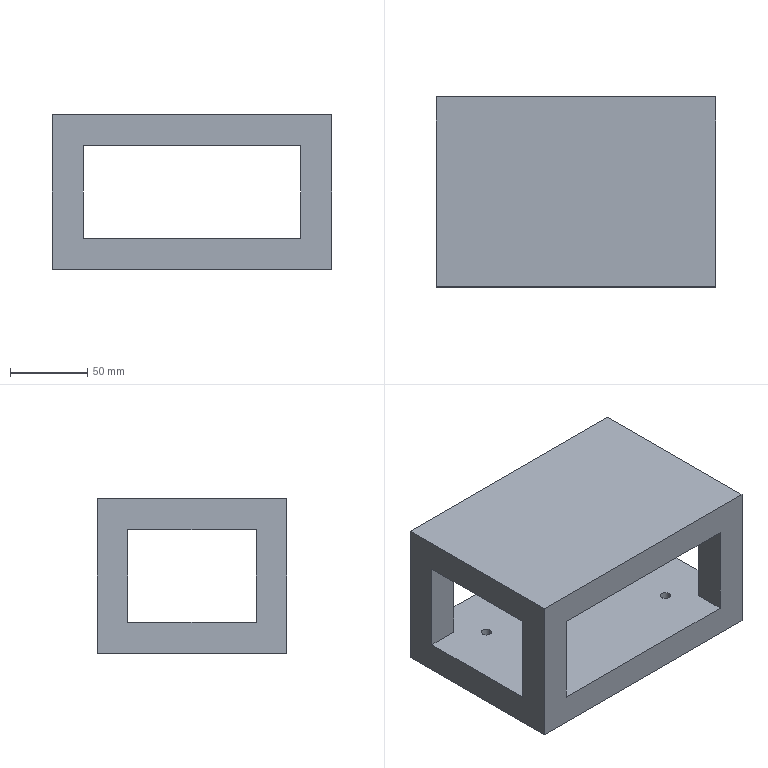Part | STEP file | ASND-0110-Body 1-24 | 1 solid | 24 faces | box 181 x 123 x 100 mm | volume 983865 mm3 | plane 16 | cylinder 8 | commonest cylinder face diameters 6.5 x8